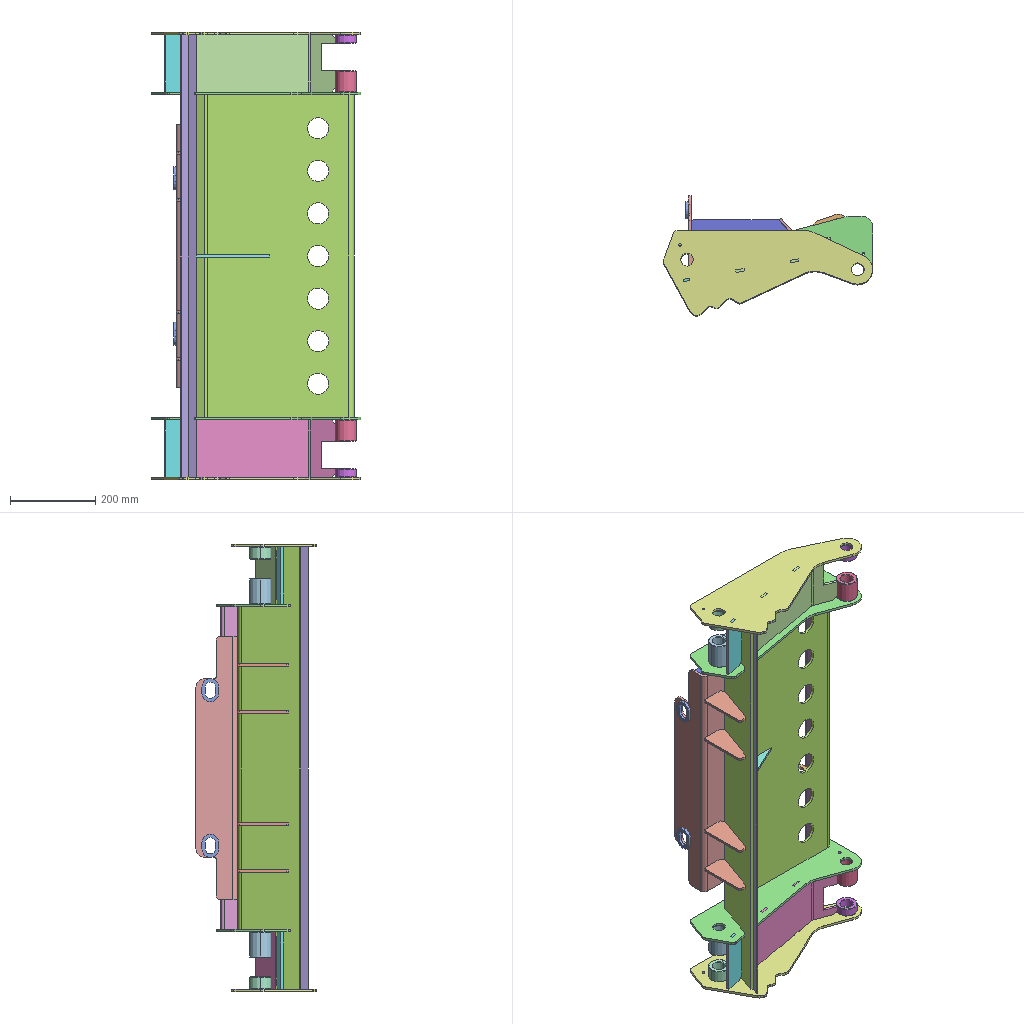Assembly | SolidWorks | 18 different items | 30 placed | box 492 x 283 x 1052 mm
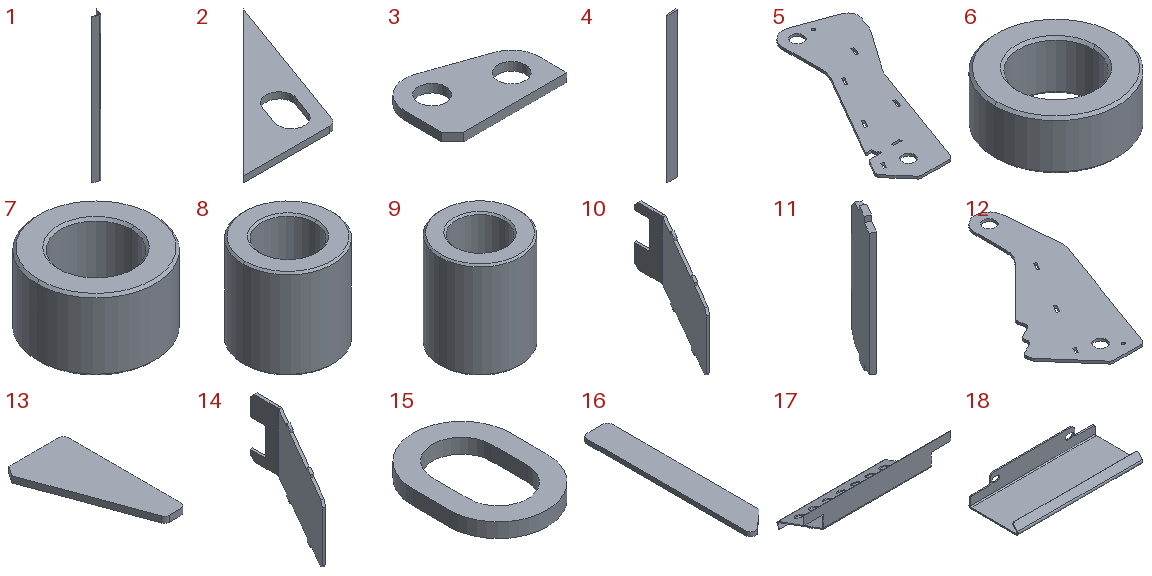Parts list (item | quantity | size | volume | features):
1 | x1 | 49.987 x 35.42 x 758 mm | 164206 mm3 | features FlatPattern 1, SMBaseFlange 1, SheetMetal 1
2 | x1 | 141.303 x 140.954 x 6 mm | 31713 mm3 | features FlatPattern 1, SMBaseFlange 1, SheetMetal 1
3 | x1 | 82.426 x 55 x 6 mm | 18808 mm3 | features FlatPattern 1, SMBaseFlange 1, SheetMetal 1
4 | x1 | 75 x 12 x 1040 mm | 832000 mm3 | features FlatPattern 1, SMBaseFlange 1, SheetMetal 1
5 | x2 | 310.123 x 471.04 x 6 mm | 332793 mm3 | features Fillet 3, FlatPattern 1, HoleWzd 1, SMBaseFlange 1, SheetMetal 1
6 | x2 | 50 x 50 x 20 mm | 24881 mm3 | features Chamfer 1, Extrusion 1
7 | x2 | 50 x 50 x 30 mm | 37448 mm3 | features Chamfer 1, Extrusion 1
8 | x2 | 50 x 50 x 50 mm | 62581 mm3 | features Chamfer 1, Extrusion 1
9 | x2 | 50 x 50 x 60 mm | 75147 mm3 | features Chamfer 1, Extrusion 1
10 | x1 | 145.088 x 308.559 x 147 mm | 266913 mm3 | features SMBaseFlange 2, Chamfer 1, Cut 1, FlatPattern 1, SheetMetal 1
11 | x2 | 31.874 x 49.208 x 147 mm | 43699 mm3 | features SMBaseFlange 2, Chamfer 1, FlatPattern 1, SheetMetal 1
12 | x2 | 278.099 x 471.04 x 6 mm | 357826 mm3 | features Fillet 2, FlatPattern 1, HoleWzd 1, SMBaseFlange 1, SheetMetal 1
13 | x4 | 59.933 x 120 x 6 mm | 29531 mm3 | features FlatPattern 1, SMBaseFlange 1, SheetMetal 1
14 | x1 | 145.088 x 308.559 x 147 mm | 266913 mm3 | features SMBaseFlange 2, Chamfer 1, Cut 1, FlatPattern 1, SheetMetal 1
15 | x2 | 40 x 55 x 6 mm | 6265 mm3 | features FlatPattern 1, SMBaseFlange 1, SheetMetal 1
16 | x2 | 34.572 x 229.825 x 6 mm | 45739 mm3 | features FlatPattern 1, SMBaseFlange 1, SheetMetal 1
17 | x1 | 1040 x 330.948 x 311.993 mm | 2463441 mm3 | features SMBaseFlange 3, ICE 2, FlatPattern 1, SheetMetal 1
18 | x1 | 620 x 243.695 x 98.004 mm | 1326121 mm3 | features SM3dBend 2, Fillet 1, FlatPattern 1, SMBaseFlange 1, SheetMetal 1
Mates (type | each side: item.copy, entity, surface, feature):
Coincident | 18.1 face plane Base-Flange1 | 15.1 face plane Base-Flange1
Concentric | 18.1 face cylinder Base-Flange1 | 15.1 face cylinder Base-Flange1 | 2 times
Concentric | 18.1 face cylinder Base-Flange1 | 15.2 face cylinder Base-Flange1 | 2 times
Coincident | 18.1 face plane Base-Flange1 | 15.2 face plane Base-Flange1
Coincident | 18.1 face plane Base-Flange1 | 17.1 face plane Base-Flange1
DistanceDim | 18.1 face plane Base-Flange1 | 17.1 face plane Cut-Extrude1
DistanceDim | 18.1 face plane Base-Flange1 | 17.1 edge
InPlace | 17.1 face plane Cut-Extrude1 | 1.1 plane
Coincident | 17.1 face plane Base-Flange1 | 2.1 face plane Base-Flange1 | 2 times
DistanceDim | 17.1 face plane Cut-Extrude1 | 2.1 face plane Base-Flange1
Coincident | 17.1 face plane Base-Flange1 | 3.1 face plane Base-Flange1
Coincident | 1.1 face plane Base-Flange1 | 3.1 face plane Base-Flange1
DistanceDim | 3.1 face plane Base-Flange1 | 17.1 face plane Cut-Extrude1
InPlace | 17.1 face plane Base-Flange1 | 4.1 plane
InPlace | 17.1 face plane Cut-Extrude1 | 5.1 plane
Concentric | 5.1 face cylinder Base-Flange1 | 8.1 face cylinder Boss-Extrude1
Coincident | 5.1 face plane Base-Flange1 | 8.1 face plane Boss-Extrude1
Coincident | 5.1 face plane Base-Flange1 | 9.1 face plane Boss-Extrude1
Concentric | 5.1 face cylinder Base-Flange1 | 9.1 face cylinder Boss-Extrude1
InPlace | 17.1 face plane Base-Flange1 | 12.1 plane
Concentric | 12.1 face cylinder Base-Flange1 | 6.1 face cylinder Boss-Extrude1
Coincident | 12.1 face plane Base-Flange1 | 6.1 face plane Boss-Extrude1
Concentric | 12.1 face cylinder Base-Flange1 | 7.1 face cylinder Boss-Extrude1
Coincident | 12.1 face plane Base-Flange1 | 7.1 face plane Boss-Extrude1
InPlace | 13.1 plane | assembly plane
Coincident | 18.1 face plane Base-Flange1 | 16.1 face plane Base-Flange1 | 2 times
DistanceDim | 16.1 face plane Base-Flange1 | 18.1 face plane Base-Flange1
Coincident | 5.2 face plane Base-Flange1 | 14.1 face plane Base-Flange1
Coincident | 5.1 face plane Base-Flange1 | 10.1 face plane Base-Flange1 | 2 times
Coincident | 12.1 face plane Base-Flange1 | 10.1 face plane Base flange 1
Coincident | 12.2 face plane Base-Flange1 | 11.1 face plane Base-Flange1 | 2 times
Coincident | 12.2 face plane Base-Flange1 | 11.1 face plane Base flange 1